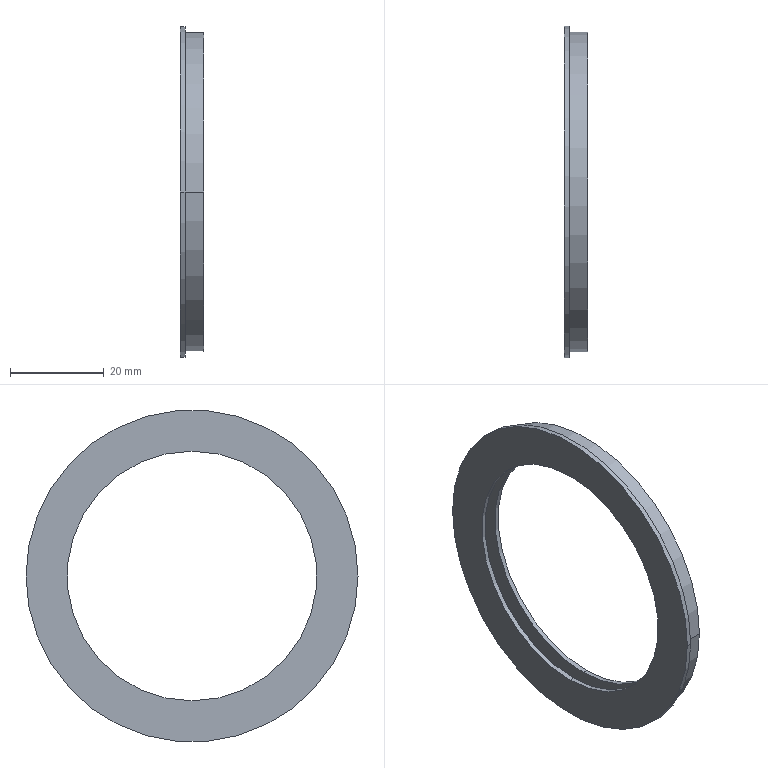Part | SolidWorks | features BaseBody 1 | 1 solid | 15 faces | box 4.95 x 70.89 x 70.89 mm | volume 3449 mm3 | spline 6 | plane 5 | cylinder 4 | commonest cylinder face diameters 68.3 x2 70.89 x2
STEP:
#1=CARTESIAN_POINT('',(14.05,40.85,49.2));
#2=VERTEX_POINT('',#1);
#3=CARTESIAN_POINT('',(14.05,109.15,49.2));
#4=VERTEX_POINT('',#3);
#5=CARTESIAN_POINT('',(14.05,75.,49.2));
#6=DIRECTION('',(-1.,0.,0.));
#7=DIRECTION('',(0.,0.,1.));
#8=AXIS2_PLACEMENT_3D('',#5,#6,#7);
#9=CIRCLE('',#8,34.15);
#10=EDGE_CURVE('',#2,#4,#9,.T.);
#11=ORIENTED_EDGE('',*,*,#10,.T.);
#12=CARTESIAN_POINT('',(10.1,109.15,49.2));
#13=VERTEX_POINT('',#12);
#14=CARTESIAN_POINT('',(12.075,109.15,49.2));
#15=DIRECTION('',(-1.,0.,0.));
#16=VECTOR('',#15,1000.);
#17=LINE('',#14,#16);
#18=EDGE_CURVE('',#4,#13,#17,.T.);
#19=ORIENTED_EDGE('',*,*,#18,.T.);
#20=CARTESIAN_POINT('',(10.1,40.85,49.2));
#21=VERTEX_POINT('',#20);
#22=CARTESIAN_POINT('',(10.1,75.,49.2));
#23=DIRECTION('',(-1.,0.,0.));
#24=DIRECTION('',(0.,0.,1.));
#25=AXIS2_PLACEMENT_3D('',#22,#23,#24);
#26=CIRCLE('',#25,34.15);
#27=EDGE_CURVE('',#21,#13,#26,.T.);
#28=ORIENTED_EDGE('',*,*,#27,.F.);
#29=CARTESIAN_POINT('',(12.075,40.85,49.2));
#30=DIRECTION('',(-1.,0.,0.));
#31=VECTOR('',#30,1000.);
#32=LINE('',#29,#31);
#33=EDGE_CURVE('',#2,#21,#32,.T.);
#34=ORIENTED_EDGE('',*,*,#33,.F.);
#35=EDGE_LOOP('',(#11,#19,#28,#34));
#36=FACE_OUTER_BOUND('',#35,.T.);
#37=CARTESIAN_POINT('',(12.075,75.,49.2));
#38=DIRECTION('',(-1.,0.,0.));
#39=DIRECTION('',(0.,-1.,0.));
#40=AXIS2_PLACEMENT_3D('',#37,#38,#39);
#41=CYLINDRICAL_SURFACE('',#40,34.15);
#42=ADVANCED_FACE('',(#36),#41,.T.);
#43=CARTESIAN_POINT('',(10.1,39.555,49.2));
#44=VERTEX_POINT('',#43);
#45=CARTESIAN_POINT('',(10.1,110.445,49.2));
#46=VERTEX_POINT('',#45);
#47=CARTESIAN_POINT('',(10.1,75.,49.2));
#48=DIRECTION('',(-1.,0.,0.));
#49=DIRECTION('',(0.,0.,1.));
#50=AXIS2_PLACEMENT_3D('',#47,#48,#49);
#51=CIRCLE('',#50,35.445);
#52=EDGE_CURVE('',#44,#46,#51,.T.);
#53=ORIENTED_EDGE('',*,*,#52,.T.);
#54=CARTESIAN_POINT('',(9.1,110.445,49.2));
#55=VERTEX_POINT('',#54);
#56=CARTESIAN_POINT('',(9.6,110.445,49.2));
#57=DIRECTION('',(-1.,0.,0.));
#58=VECTOR('',#57,1000.);
#59=LINE('',#56,#58);
#60=EDGE_CURVE('',#46,#55,#59,.T.);
#61=ORIENTED_EDGE('',*,*,#60,.T.);
#62=CARTESIAN_POINT('',(9.1,39.555,49.2));
#63=VERTEX_POINT('',#62);
#64=CARTESIAN_POINT('',(9.1,75.,49.2));
#65=DIRECTION('',(-1.,0.,0.));
#66=DIRECTION('',(0.,0.,1.));
#67=AXIS2_PLACEMENT_3D('',#64,#65,#66);
#68=CIRCLE('',#67,35.445);
#69=EDGE_CURVE('',#63,#55,#68,.T.);
#70=ORIENTED_EDGE('',*,*,#69,.F.);
#71=CARTESIAN_POINT('',(9.6,39.555,49.2));
#72=DIRECTION('',(-1.,0.,0.));
#73=VECTOR('',#72,1000.);
#74=LINE('',#71,#73);
#75=EDGE_CURVE('',#44,#63,#74,.T.);
#76=ORIENTED_EDGE('',*,*,#75,.F.);
#77=EDGE_LOOP('',(#53,#61,#70,#76));
#78=FACE_OUTER_BOUND('',#77,.T.);
#79=CARTESIAN_POINT('',(9.6,75.,49.2));
#80=DIRECTION('',(-1.,0.,0.));
#81=DIRECTION('',(0.,-1.,0.));
#82=AXIS2_PLACEMENT_3D('',#79,#80,#81);
#83=CYLINDRICAL_SURFACE('',#82,35.445);
#84=ADVANCED_FACE('',(#78),#83,.T.);
#85=CARTESIAN_POINT('',(10.1,75.,22.55));
#86=VERTEX_POINT('',#85);
#87=CARTESIAN_POINT('',(10.1,75.,75.85));
#88=VERTEX_POINT('',#87);
#89=CARTESIAN_POINT('',(10.1,75.,49.2));
#90=DIRECTION('',(-1.,0.,0.));
#91=DIRECTION('',(0.,0.,1.));
#92=AXIS2_PLACEMENT_3D('',#89,#90,#91);
#93=CIRCLE('',#92,26.65);
#94=EDGE_CURVE('',#86,#88,#93,.T.);
#95=ORIENTED_EDGE('',*,*,#94,.F.);
#96=CARTESIAN_POINT('',(9.1,75.,22.55));
#97=VERTEX_POINT('',#96);
#98=CARTESIAN_POINT('',(9.6,75.,22.55));
#99=DIRECTION('',(-1.,0.,0.));
#100=VECTOR('',#99,1000.);
#101=LINE('',#98,#100);
#102=EDGE_CURVE('',#86,#97,#101,.T.);
#103=ORIENTED_EDGE('',*,*,#102,.T.);
#104=CARTESIAN_POINT('',(9.1,75.,75.85));
#105=VERTEX_POINT('',#104);
#106=CARTESIAN_POINT('',(9.1,75.,49.2));
#107=DIRECTION('',(-1.,0.,0.));
#108=DIRECTION('',(0.,0.,1.));
#109=AXIS2_PLACEMENT_3D('',#106,#107,#108);
#110=CIRCLE('',#109,26.65);
#111=EDGE_CURVE('',#97,#105,#110,.T.);
#112=ORIENTED_EDGE('',*,*,#111,.T.);
#113=CARTESIAN_POINT('',(9.6,75.,75.85));
#114=DIRECTION('',(-1.,0.,0.));
#115=VECTOR('',#114,1000.);
#116=LINE('',#113,#115);
#117=EDGE_CURVE('',#88,#105,#116,.T.);
#118=ORIENTED_EDGE('',*,*,#117,.F.);
#119=EDGE_LOOP('',(#95,#103,#112,#118));
#120=FACE_OUTER_BOUND('',#119,.T.);
#121=CARTESIAN_POINT('',(10.1,75.,75.85));
#122=CARTESIAN_POINT('',(9.1,75.,75.85));
#123=CARTESIAN_POINT('',(10.1,21.7,75.85));
#124=CARTESIAN_POINT('',(9.1,21.7,75.85));
#125=CARTESIAN_POINT('',(10.1,21.7,22.55));
#126=CARTESIAN_POINT('',(9.1,21.7,22.55));
#127=CARTESIAN_POINT('',(10.1,75.,22.55));
#128=CARTESIAN_POINT('',(9.1,75.,22.55));
#129=(BOUNDED_SURFACE()B_SPLINE_SURFACE(3,1,((#121,#122),(#123,#124),(#125,#126),(#127,#128)),.UNSPECIFIED.,.F.,.F.,.F.)B_SPLINE_SURFACE_WITH_KNOTS((4,4),(2,2),(0.,1.),(0.,1.),.UNSPECIFIED.)GEOMETRIC_REPRESENTATION_ITEM()RATIONAL_B_SPLINE_SURFACE(((1.,1.),(0.3333,0.3333),(0.3333,0.3333),(1.,1.)))REPRESENTATION_ITEM('')SURFACE());
#130=ADVANCED_FACE('',(#120),#129,.T.);
#131=CARTESIAN_POINT('',(13.06,75.,15.55));
#132=VERTEX_POINT('',#131);
#133=CARTESIAN_POINT('',(13.06,75.,82.85));
#134=VERTEX_POINT('',#133);
#135=CARTESIAN_POINT('',(13.06,75.,49.2));
#136=DIRECTION('',(-1.,0.,0.));
#137=DIRECTION('',(0.,0.,1.));
#138=AXIS2_PLACEMENT_3D('',#135,#136,#137);
#139=CIRCLE('',#138,33.65);
#140=EDGE_CURVE('',#132,#134,#139,.T.);
#141=ORIENTED_EDGE('',*,*,#140,.F.);
#142=CARTESIAN_POINT('',(10.1,75.,15.55));
#143=VERTEX_POINT('',#142);
#144=CARTESIAN_POINT('',(11.58,75.,15.55));
#145=DIRECTION('',(-1.,0.,0.));
#146=VECTOR('',#145,1000.);
#147=LINE('',#144,#146);
#148=EDGE_CURVE('',#132,#143,#147,.T.);
#149=ORIENTED_EDGE('',*,*,#148,.T.);
#150=CARTESIAN_POINT('',(10.1,75.,82.85));
#151=VERTEX_POINT('',#150);
#152=CARTESIAN_POINT('',(10.1,75.,49.2));
#153=DIRECTION('',(-1.,0.,0.));
#154=DIRECTION('',(0.,0.,1.));
#155=AXIS2_PLACEMENT_3D('',#152,#153,#154);
#156=CIRCLE('',#155,33.65);
#157=EDGE_CURVE('',#143,#151,#156,.T.);
#158=ORIENTED_EDGE('',*,*,#157,.T.);
#159=CARTESIAN_POINT('',(11.58,75.,82.85));
#160=DIRECTION('',(-1.,0.,0.));
#161=VECTOR('',#160,1000.);
#162=LINE('',#159,#161);
#163=EDGE_CURVE('',#134,#151,#162,.T.);
#164=ORIENTED_EDGE('',*,*,#163,.F.);
#165=EDGE_LOOP('',(#141,#149,#158,#164));
#166=FACE_OUTER_BOUND('',#165,.T.);
#167=CARTESIAN_POINT('',(13.06,75.,82.85));
#168=CARTESIAN_POINT('',(10.1,75.,82.85));
#169=CARTESIAN_POINT('',(13.06,7.7,82.85));
#170=CARTESIAN_POINT('',(10.1,7.7,82.85));
#171=CARTESIAN_POINT('',(13.06,7.7,15.55));
#172=CARTESIAN_POINT('',(10.1,7.7,15.55));
#173=CARTESIAN_POINT('',(13.06,75.,15.55));
#174=CARTESIAN_POINT('',(10.1,75.,15.55));
#175=(BOUNDED_SURFACE()B_SPLINE_SURFACE(3,1,((#167,#168),(#169,#170),(#171,#172),(#173,#174)),.UNSPECIFIED.,.F.,.F.,.F.)B_SPLINE_SURFACE_WITH_KNOTS((4,4),(2,2),(0.,1.),(0.,1.),.UNSPECIFIED.)GEOMETRIC_REPRESENTATION_ITEM()RATIONAL_B_SPLINE_SURFACE(((1.,1.),(0.3333,0.3333),(0.3333,0.3333),(1.,1.)))REPRESENTATION_ITEM('')SURFACE());
#176=ADVANCED_FACE('',(#166),#175,.T.);
#177=CARTESIAN_POINT('',(14.05,75.,22.55));
#178=VERTEX_POINT('',#177);
#179=CARTESIAN_POINT('',(14.05,75.,75.85));
#180=VERTEX_POINT('',#179);
#181=CARTESIAN_POINT('',(14.05,75.,49.2));
#182=DIRECTION('',(-1.,0.,0.));
#183=DIRECTION('',(0.,0.,1.));
#184=AXIS2_PLACEMENT_3D('',#181,#182,#183);
#185=CIRCLE('',#184,26.65);
#186=EDGE_CURVE('',#178,#180,#185,.T.);
#187=ORIENTED_EDGE('',*,*,#186,.F.);
#188=CARTESIAN_POINT('',(13.06,75.,22.55));
#189=VERTEX_POINT('',#188);
#190=CARTESIAN_POINT('',(13.555,75.,22.55));
#191=DIRECTION('',(-1.,0.,0.));
#192=VECTOR('',#191,1000.);
#193=LINE('',#190,#192);
#194=EDGE_CURVE('',#178,#189,#193,.T.);
#195=ORIENTED_EDGE('',*,*,#194,.T.);
#196=CARTESIAN_POINT('',(13.06,75.,75.85));
#197=VERTEX_POINT('',#196);
#198=CARTESIAN_POINT('',(13.06,75.,49.2));
#199=DIRECTION('',(-1.,0.,0.));
#200=DIRECTION('',(0.,0.,1.));
#201=AXIS2_PLACEMENT_3D('',#198,#199,#200);
#202=CIRCLE('',#201,26.65);
#203=EDGE_CURVE('',#189,#197,#202,.T.);
#204=ORIENTED_EDGE('',*,*,#203,.T.);
#205=CARTESIAN_POINT('',(13.555,75.,75.85));
#206=DIRECTION('',(-1.,0.,0.));
#207=VECTOR('',#206,1000.);
#208=LINE('',#205,#207);
#209=EDGE_CURVE('',#180,#197,#208,.T.);
#210=ORIENTED_EDGE('',*,*,#209,.F.);
#211=EDGE_LOOP('',(#187,#195,#204,#210));
#212=FACE_OUTER_BOUND('',#211,.T.);
#213=CARTESIAN_POINT('',(14.05,75.,75.85));
#214=CARTESIAN_POINT('',(13.06,75.,75.85));
#215=CARTESIAN_POINT('',(14.05,21.7,75.85));
#216=CARTESIAN_POINT('',(13.06,21.7,75.85));
#217=CARTESIAN_POINT('',(14.05,21.7,22.55));
#218=CARTESIAN_POINT('',(13.06,21.7,22.55));
#219=CARTESIAN_POINT('',(14.05,75.,22.55));
#220=CARTESIAN_POINT('',(13.06,75.,22.55));
#221=(BOUNDED_SURFACE()B_SPLINE_SURFACE(3,1,((#213,#214),(#215,#216),(#217,#218),(#219,#220)),.UNSPECIFIED.,.F.,.F.,.F.)B_SPLINE_SURFACE_WITH_KNOTS((4,4),(2,2),(0.,1.),(0.,1.),.UNSPECIFIED.)GEOMETRIC_REPRESENTATION_ITEM()RATIONAL_B_SPLINE_SURFACE(((1.,1.),(0.3333,0.3333),(0.3333,0.3333),(1.,1.)))REPRESENTATION_ITEM('')SURFACE());
#222=ADVANCED_FACE('',(#212),#221,.T.);
#223=CARTESIAN_POINT('',(14.05,75.,49.2));
#224=DIRECTION('',(-1.,0.,0.));
#225=DIRECTION('',(0.,0.,1.));
#226=AXIS2_PLACEMENT_3D('',#223,#224,#225);
#227=CIRCLE('',#226,26.65);
#228=EDGE_CURVE('',#180,#178,#227,.T.);
#229=ORIENTED_EDGE('',*,*,#228,.T.);
#230=ORIENTED_EDGE('',*,*,#186,.T.);
#231=EDGE_LOOP('',(#229,#230));
#232=FACE_BOUND('',#231,.T.);
#233=ORIENTED_EDGE('',*,*,#10,.F.);
#234=CARTESIAN_POINT('',(14.05,75.,49.2));
#235=DIRECTION('',(-1.,0.,0.));
#236=DIRECTION('',(0.,0.,1.));
#237=AXIS2_PLACEMENT_3D('',#234,#235,#236);
#238=CIRCLE('',#237,34.15);
#239=EDGE_CURVE('',#4,#2,#238,.T.);
#240=ORIENTED_EDGE('',*,*,#239,.F.);
#241=EDGE_LOOP('',(#233,#240));
#242=FACE_OUTER_BOUND('',#241,.T.);
#243=CARTESIAN_POINT('',(14.05,75.,79.6));
#244=DIRECTION('',(1.,0.,0.));
#245=DIRECTION('',(0.,1.,0.));
#246=AXIS2_PLACEMENT_3D('',#243,#244,#245);
#247=PLANE('',#246);
#248=ADVANCED_FACE('',(#232,#242),#247,.T.);
#249=ORIENTED_EDGE('',*,*,#194,.F.);
#250=ORIENTED_EDGE('',*,*,#228,.F.);
#251=ORIENTED_EDGE('',*,*,#209,.T.);
#252=CARTESIAN_POINT('',(13.06,75.,49.2));
#253=DIRECTION('',(-1.,0.,0.));
#254=DIRECTION('',(0.,0.,1.));
#255=AXIS2_PLACEMENT_3D('',#252,#253,#254);
#256=CIRCLE('',#255,26.65);
#257=EDGE_CURVE('',#197,#189,#256,.T.);
#258=ORIENTED_EDGE('',*,*,#257,.T.);
#259=EDGE_LOOP('',(#249,#250,#251,#258));
#260=FACE_OUTER_BOUND('',#259,.T.);
#261=CARTESIAN_POINT('',(14.05,75.,22.55));
#262=CARTESIAN_POINT('',(13.06,75.,22.55));
#263=CARTESIAN_POINT('',(14.05,128.3,22.55));
#264=CARTESIAN_POINT('',(13.06,128.3,22.55));
#265=CARTESIAN_POINT('',(14.05,128.3,75.85));
#266=CARTESIAN_POINT('',(13.06,128.3,75.85));
#267=CARTESIAN_POINT('',(14.05,75.,75.85));
#268=CARTESIAN_POINT('',(13.06,75.,75.85));
#269=(BOUNDED_SURFACE()B_SPLINE_SURFACE(3,1,((#261,#262),(#263,#264),(#265,#266),(#267,#268)),.UNSPECIFIED.,.F.,.F.,.F.)B_SPLINE_SURFACE_WITH_KNOTS((4,4),(2,2),(0.,1.),(0.,1.),.UNSPECIFIED.)GEOMETRIC_REPRESENTATION_ITEM()RATIONAL_B_SPLINE_SURFACE(((1.,1.),(0.3333,0.3333),(0.3333,0.3333),(1.,1.)))REPRESENTATION_ITEM('')SURFACE());
#270=ADVANCED_FACE('',(#260),#269,.T.);
#271=CARTESIAN_POINT('',(13.06,75.,49.2));
#272=DIRECTION('',(-1.,0.,0.));
#273=DIRECTION('',(0.,0.,1.));
#274=AXIS2_PLACEMENT_3D('',#271,#272,#273);
#275=CIRCLE('',#274,33.65);
#276=EDGE_CURVE('',#134,#132,#275,.T.);
#277=ORIENTED_EDGE('',*,*,#276,.T.);
#278=ORIENTED_EDGE('',*,*,#140,.T.);
#279=EDGE_LOOP('',(#277,#278));
#280=FACE_OUTER_BOUND('',#279,.T.);
#281=ORIENTED_EDGE('',*,*,#257,.F.);
#282=ORIENTED_EDGE('',*,*,#203,.F.);
#283=EDGE_LOOP('',(#281,#282));
#284=FACE_BOUND('',#283,.T.);
#285=CARTESIAN_POINT('',(13.06,75.,79.35));
#286=DIRECTION('',(-1.,0.,0.));
#287=DIRECTION('',(0.,-1.,0.));
#288=AXIS2_PLACEMENT_3D('',#285,#286,#287);
#289=PLANE('',#288);
#290=ADVANCED_FACE('',(#280,#284),#289,.T.);
#291=ORIENTED_EDGE('',*,*,#148,.F.);
#292=ORIENTED_EDGE('',*,*,#276,.F.);
#293=ORIENTED_EDGE('',*,*,#163,.T.);
#294=CARTESIAN_POINT('',(10.1,75.,49.2));
#295=DIRECTION('',(-1.,0.,0.));
#296=DIRECTION('',(0.,0.,1.));
#297=AXIS2_PLACEMENT_3D('',#294,#295,#296);
#298=CIRCLE('',#297,33.65);
#299=EDGE_CURVE('',#151,#143,#298,.T.);
#300=ORIENTED_EDGE('',*,*,#299,.T.);
#301=EDGE_LOOP('',(#291,#292,#293,#300));
#302=FACE_OUTER_BOUND('',#301,.T.);
#303=CARTESIAN_POINT('',(13.06,75.,15.55));
#304=CARTESIAN_POINT('',(10.1,75.,15.55));
#305=CARTESIAN_POINT('',(13.06,142.3,15.55));
#306=CARTESIAN_POINT('',(10.1,142.3,15.55));
#307=CARTESIAN_POINT('',(13.06,142.3,82.85));
#308=CARTESIAN_POINT('',(10.1,142.3,82.85));
#309=CARTESIAN_POINT('',(13.06,75.,82.85));
#310=CARTESIAN_POINT('',(10.1,75.,82.85));
#311=(BOUNDED_SURFACE()B_SPLINE_SURFACE(3,1,((#303,#304),(#305,#306),(#307,#308),(#309,#310)),.UNSPECIFIED.,.F.,.F.,.F.)B_SPLINE_SURFACE_WITH_KNOTS((4,4),(2,2),(0.,1.),(0.,1.),.UNSPECIFIED.)GEOMETRIC_REPRESENTATION_ITEM()RATIONAL_B_SPLINE_SURFACE(((1.,1.),(0.3333,0.3333),(0.3333,0.3333),(1.,1.)))REPRESENTATION_ITEM('')SURFACE());
#312=ADVANCED_FACE('',(#302),#311,.T.);
#313=CARTESIAN_POINT('',(10.1,75.,49.2));
#314=DIRECTION('',(-1.,0.,0.));
#315=DIRECTION('',(0.,0.,1.));
#316=AXIS2_PLACEMENT_3D('',#313,#314,#315);
#317=CIRCLE('',#316,26.65);
#318=EDGE_CURVE('',#88,#86,#317,.T.);
#319=ORIENTED_EDGE('',*,*,#318,.T.);
#320=ORIENTED_EDGE('',*,*,#94,.T.);
#321=EDGE_LOOP('',(#319,#320));
#322=FACE_BOUND('',#321,.T.);
#323=ORIENTED_EDGE('',*,*,#299,.F.);
#324=ORIENTED_EDGE('',*,*,#157,.F.);
#325=EDGE_LOOP('',(#323,#324));
#326=FACE_OUTER_BOUND('',#325,.T.);
#327=CARTESIAN_POINT('',(10.1,75.,79.35));
#328=DIRECTION('',(1.,0.,0.));
#329=DIRECTION('',(0.,1.,0.));
#330=AXIS2_PLACEMENT_3D('',#327,#328,#329);
#331=PLANE('',#330);
#332=ADVANCED_FACE('',(#322,#326),#331,.T.);
#333=ORIENTED_EDGE('',*,*,#102,.F.);
#334=ORIENTED_EDGE('',*,*,#318,.F.);
#335=ORIENTED_EDGE('',*,*,#117,.T.);
#336=CARTESIAN_POINT('',(9.1,75.,49.2));
#337=DIRECTION('',(-1.,0.,0.));
#338=DIRECTION('',(0.,0.,1.));
#339=AXIS2_PLACEMENT_3D('',#336,#337,#338);
#340=CIRCLE('',#339,26.65);
#341=EDGE_CURVE('',#105,#97,#340,.T.);
#342=ORIENTED_EDGE('',*,*,#341,.T.);
#343=EDGE_LOOP('',(#333,#334,#335,#342));
#344=FACE_OUTER_BOUND('',#343,.T.);
#345=CARTESIAN_POINT('',(10.1,75.,22.55));
#346=CARTESIAN_POINT('',(9.1,75.,22.55));
#347=CARTESIAN_POINT('',(10.1,128.3,22.55));
#348=CARTESIAN_POINT('',(9.1,128.3,22.55));
#349=CARTESIAN_POINT('',(10.1,128.3,75.85));
#350=CARTESIAN_POINT('',(9.1,128.3,75.85));
#351=CARTESIAN_POINT('',(10.1,75.,75.85));
#352=CARTESIAN_POINT('',(9.1,75.,75.85));
#353=(BOUNDED_SURFACE()B_SPLINE_SURFACE(3,1,((#345,#346),(#347,#348),(#349,#350),(#351,#352)),.UNSPECIFIED.,.F.,.F.,.F.)B_SPLINE_SURFACE_WITH_KNOTS((4,4),(2,2),(0.,1.),(0.,1.),.UNSPECIFIED.)GEOMETRIC_REPRESENTATION_ITEM()RATIONAL_B_SPLINE_SURFACE(((1.,1.),(0.3333,0.3333),(0.3333,0.3333),(1.,1.)))REPRESENTATION_ITEM('')SURFACE());
#354=ADVANCED_FACE('',(#344),#353,.T.);
#355=ORIENTED_EDGE('',*,*,#69,.T.);
#356=CARTESIAN_POINT('',(9.1,75.,49.2));
#357=DIRECTION('',(-1.,0.,0.));
#358=DIRECTION('',(0.,0.,1.));
#359=AXIS2_PLACEMENT_3D('',#356,#357,#358);
#360=CIRCLE('',#359,35.445);
#361=EDGE_CURVE('',#55,#63,#360,.T.);
#362=ORIENTED_EDGE('',*,*,#361,.T.);
#363=EDGE_LOOP('',(#355,#362));
#364=FACE_OUTER_BOUND('',#363,.T.);
#365=ORIENTED_EDGE('',*,*,#341,.F.);
#366=ORIENTED_EDGE('',*,*,#111,.F.);
#367=EDGE_LOOP('',(#365,#366));
#368=FACE_BOUND('',#367,.T.);
#369=CARTESIAN_POINT('',(9.1,75.,80.248));
#370=DIRECTION('',(-1.,0.,0.));
#371=DIRECTION('',(0.,-1.,0.));
#372=AXIS2_PLACEMENT_3D('',#369,#370,#371);
#373=PLANE('',#372);
#374=ADVANCED_FACE('',(#364,#368),#373,.T.);
#375=ORIENTED_EDGE('',*,*,#60,.F.);
#376=CARTESIAN_POINT('',(10.1,75.,49.2));
#377=DIRECTION('',(-1.,0.,0.));
#378=DIRECTION('',(0.,0.,1.));
#379=AXIS2_PLACEMENT_3D('',#376,#377,#378);
#380=CIRCLE('',#379,35.445);
#381=EDGE_CURVE('',#46,#44,#380,.T.);
#382=ORIENTED_EDGE('',*,*,#381,.T.);
#383=ORIENTED_EDGE('',*,*,#75,.T.);
#384=ORIENTED_EDGE('',*,*,#361,.F.);
#385=EDGE_LOOP('',(#375,#382,#383,#384));
#386=FACE_OUTER_BOUND('',#385,.T.);
#387=CARTESIAN_POINT('',(9.6,75.,49.2));
#388=DIRECTION('',(-1.,0.,0.));
#389=DIRECTION('',(0.,-1.,0.));
#390=AXIS2_PLACEMENT_3D('',#387,#388,#389);
#391=CYLINDRICAL_SURFACE('',#390,35.445);
#392=ADVANCED_FACE('',(#386),#391,.T.);
#393=ORIENTED_EDGE('',*,*,#27,.T.);
#394=CARTESIAN_POINT('',(10.1,75.,49.2));
#395=DIRECTION('',(-1.,0.,0.));
#396=DIRECTION('',(0.,0.,1.));
#397=AXIS2_PLACEMENT_3D('',#394,#395,#396);
#398=CIRCLE('',#397,34.15);
#399=EDGE_CURVE('',#13,#21,#398,.T.);
#400=ORIENTED_EDGE('',*,*,#399,.T.);
#401=EDGE_LOOP('',(#393,#400));
#402=FACE_BOUND('',#401,.T.);
#403=ORIENTED_EDGE('',*,*,#52,.F.);
#404=ORIENTED_EDGE('',*,*,#381,.F.);
#405=EDGE_LOOP('',(#403,#404));
#406=FACE_OUTER_BOUND('',#405,.T.);
#407=CARTESIAN_POINT('',(10.1,75.,83.998));
#408=DIRECTION('',(1.,0.,0.));
#409=DIRECTION('',(0.,1.,0.));
#410=AXIS2_PLACEMENT_3D('',#407,#408,#409);
#411=PLANE('',#410);
#412=ADVANCED_FACE('',(#402,#406),#411,.T.);
#413=ORIENTED_EDGE('',*,*,#18,.F.);
#414=ORIENTED_EDGE('',*,*,#239,.T.);
#415=ORIENTED_EDGE('',*,*,#33,.T.);
#416=ORIENTED_EDGE('',*,*,#399,.F.);
#417=EDGE_LOOP('',(#413,#414,#415,#416));
#418=FACE_OUTER_BOUND('',#417,.T.);
#419=CARTESIAN_POINT('',(12.075,75.,49.2));
#420=DIRECTION('',(-1.,0.,0.));
#421=DIRECTION('',(0.,-1.,0.));
#422=AXIS2_PLACEMENT_3D('',#419,#420,#421);
#423=CYLINDRICAL_SURFACE('',#422,34.15);
#424=ADVANCED_FACE('',(#418),#423,.T.);
#425=CLOSED_SHELL('',(#42,#84,#130,#176,#222,#248,#270,#290,#312,#332,#354,#374,#392,#412,#424));
#426=MANIFOLD_SOLID_BREP('',#425);
#427=CARTESIAN_POINT('',(0.,0.,0.));
#428=DIRECTION('',(0.,0.,1.));
#429=DIRECTION('',(1.,0.,0.));
#430=AXIS2_PLACEMENT_3D('',#427,#428,#429);
#431=(LENGTH_UNIT()NAMED_UNIT(*)SI_UNIT(.MILLI.,.METRE.));
#432=UNCERTAINTY_MEASURE_WITH_UNIT(LENGTH_MEASURE(0.00001),#431,'','');
#433=(NAMED_UNIT(*)PLANE_ANGLE_UNIT()SI_UNIT($,.RADIAN.));
#434=(NAMED_UNIT(*)SI_UNIT($,.STERADIAN.)SOLID_ANGLE_UNIT());
#435=(GEOMETRIC_REPRESENTATION_CONTEXT(3)GLOBAL_UNCERTAINTY_ASSIGNED_CONTEXT((#432))GLOBAL_UNIT_ASSIGNED_CONTEXT((#431,#433,#434))REPRESENTATION_CONTEXT('',''));
#436=ADVANCED_BREP_SHAPE_REPRESENTATION('',(#426,#430),#435);